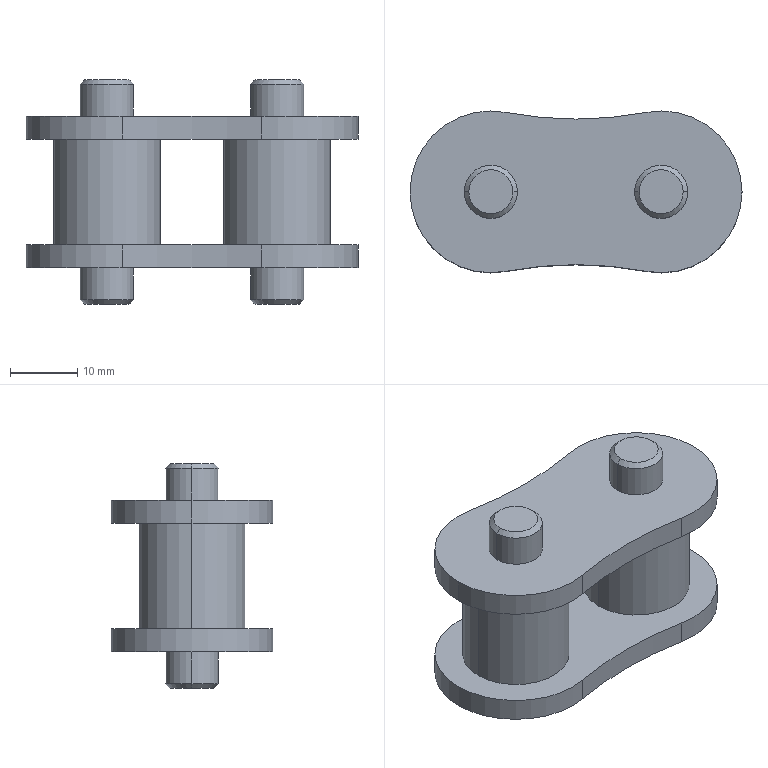Part | STEP file | 1 solid | 38 faces | box 49.53 x 24.13 x 33.5 mm | volume 14381 mm3 | cylinder 22 | cone 8 | plane 8 | commonest cylinder face diameters 7.94 x8 24.13 x6 15.88 x4 110.761 x4